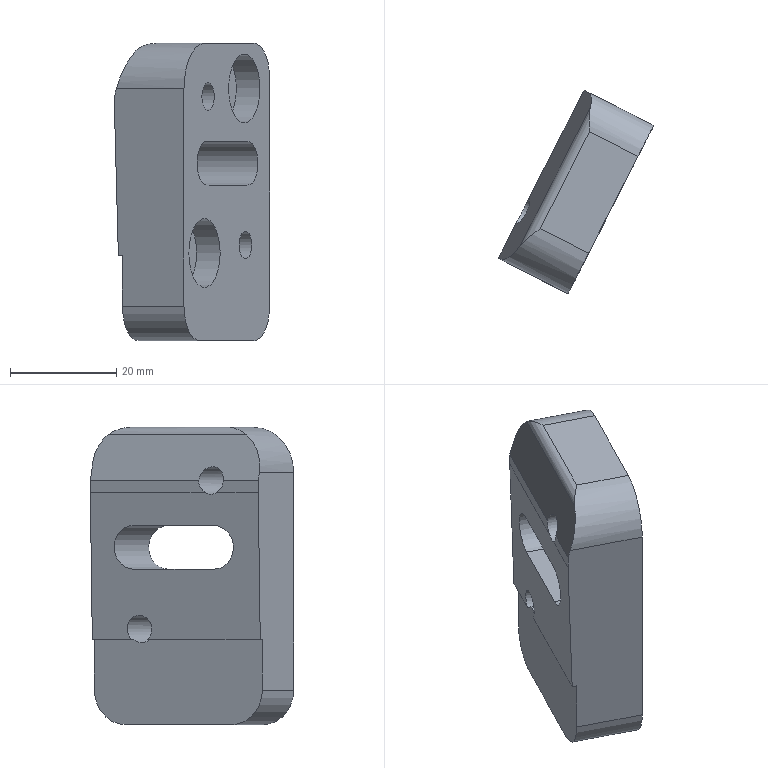Part | STEP file | gslz 2016.10.28-13_id1786_x_t | 1 solid | 27 faces | box 29.214 x 38.304 x 56 mm | volume 22057 mm3 | plane 16 | cylinder 9 | spline 2 | commonest cylinder face diameters 13 x5 5.2 x2 4 x1 17 x1